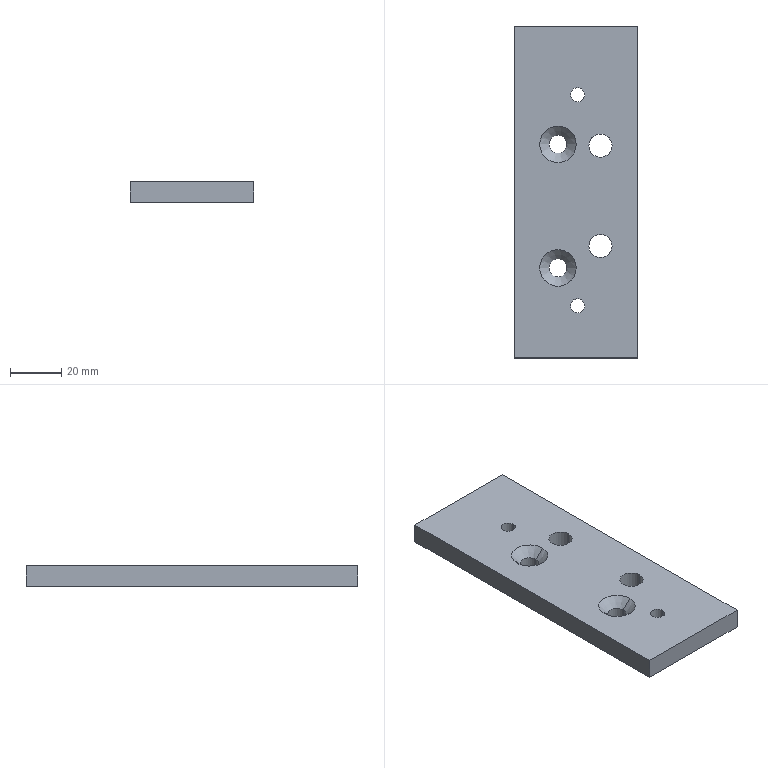Part | 1 solid | 22 faces | box 48 x 129 x 8 mm | volume 47140 mm3 | cylinder 12 | plane 6 | cone 4 | commonest cylinder face diameters 5.5 x4 7 x4 9 x4